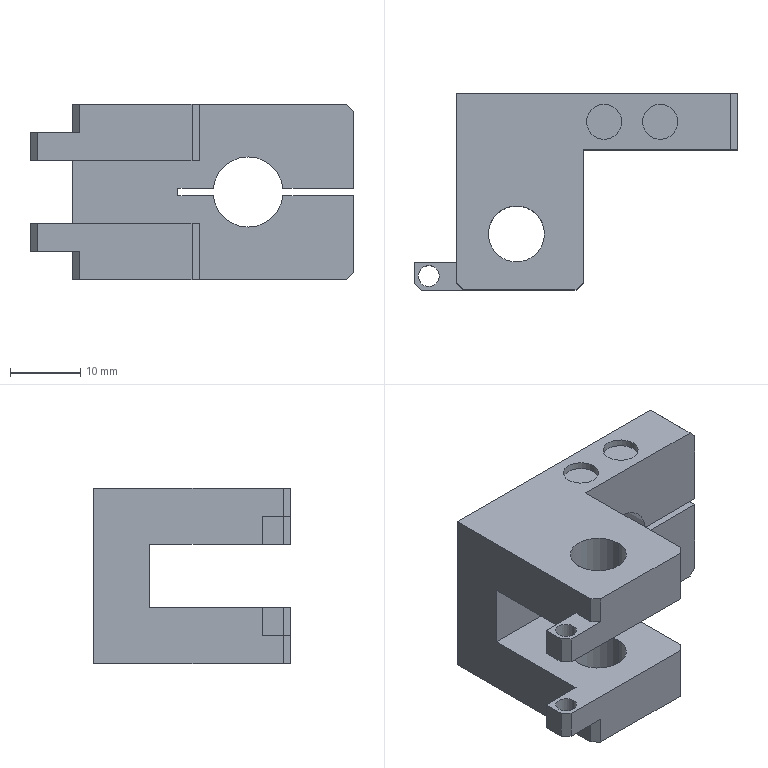Part | SolidWorks | features ICE 8, Chamfer 2, Extrusion 1 | 1 solid | 55 faces | box 46 x 28 x 25 mm | volume 12240 mm3 | plane 36 | cylinder 19 | commonest cylinder face diameters 5 x8 3 x4 8 x4 10 x3